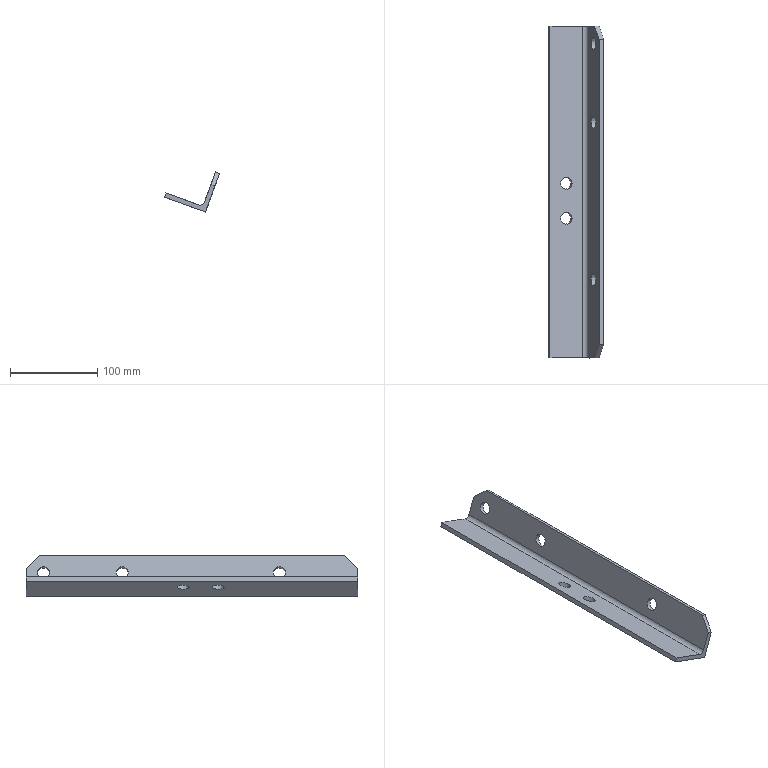Part | NX | features solid 2 | 1 solid | 16 faces | box 63.06 x 380 x 45.876 mm | volume 171865 mm3 | plane 10 | cylinder 6 | commonest cylinder face diameters 14 x5 10 x1
STEP:
#1=CARTESIAN_POINT('',(-698.232,780.,85.667));
#2=VERTEX_POINT('',#1);
#3=CARTESIAN_POINT('',(-695.838,780.,92.245));
#4=DIRECTION('',(-0.9397,0.,0.342));
#5=DIRECTION('',(-0.342,0.,-0.9397));
#6=AXIS2_PLACEMENT_3D('',#3,#4,#5);
#7=CIRCLE('',#6,7.);
#8=EDGE_CURVE('',#2,#2,#7,.F.);
#9=ORIENTED_EDGE('',*,*,#8,.T.);
#10=EDGE_LOOP('',(#9));
#11=FACE_BOUND('',#10,.T.);
#12=CARTESIAN_POINT('',(-698.232,960.,85.667));
#13=VERTEX_POINT('',#12);
#14=CARTESIAN_POINT('',(-695.838,960.,92.245));
#15=DIRECTION('',(-0.9397,0.,0.342));
#16=DIRECTION('',(-0.342,0.,-0.9397));
#17=AXIS2_PLACEMENT_3D('',#14,#15,#16);
#18=CIRCLE('',#17,7.);
#19=EDGE_CURVE('',#13,#13,#18,.F.);
#20=ORIENTED_EDGE('',*,*,#19,.T.);
#21=EDGE_LOOP('',(#20));
#22=FACE_BOUND('',#21,.T.);
#23=CARTESIAN_POINT('',(-694.127,1070.,96.944));
#24=VERTEX_POINT('',#23);
#25=CARTESIAN_POINT('',(-701.652,1070.,76.27));
#26=VERTEX_POINT('',#25);
#27=CARTESIAN_POINT('',(-693.101,1070.,99.763));
#28=DIRECTION('',(-0.342,0.,-0.9397));
#29=VECTOR('',#28,1000.);
#30=LINE('',#27,#29);
#31=EDGE_CURVE('',#24,#26,#30,.T.);
#32=ORIENTED_EDGE('',*,*,#31,.T.);
#33=CARTESIAN_POINT('',(-701.652,690.,76.27));
#34=VERTEX_POINT('',#33);
#35=CARTESIAN_POINT('',(-701.652,1109.813,76.27));
#36=DIRECTION('',(0.,1.,0.));
#37=VECTOR('',#36,1000.);
#38=LINE('',#35,#37);
#39=EDGE_CURVE('',#34,#26,#38,.T.);
#40=ORIENTED_EDGE('',*,*,#39,.F.);
#41=CARTESIAN_POINT('',(-694.127,690.,96.944));
#42=VERTEX_POINT('',#41);
#43=CARTESIAN_POINT('',(-695.838,690.,92.245));
#44=DIRECTION('',(0.342,0.,0.9397));
#45=VECTOR('',#44,1000.);
#46=LINE('',#43,#45);
#47=EDGE_CURVE('',#34,#42,#46,.T.);
#48=ORIENTED_EDGE('',*,*,#47,.T.);
#49=CARTESIAN_POINT('',(-688.997,705.,111.039));
#50=VERTEX_POINT('',#49);
#51=CARTESIAN_POINT('',(-670.59,758.818,161.611));
#52=DIRECTION('',(0.2418,0.7071,0.6645));
#53=VECTOR('',#52,1000.);
#54=LINE('',#51,#53);
#55=EDGE_CURVE('',#50,#42,#54,.F.);
#56=ORIENTED_EDGE('',*,*,#55,.F.);
#57=CARTESIAN_POINT('',(-688.997,1055.,111.039));
#58=VERTEX_POINT('',#57);
#59=CARTESIAN_POINT('',(-688.997,894.636,111.039));
#60=DIRECTION('',(0.,1.,0.));
#61=VECTOR('',#60,1000.);
#62=LINE('',#59,#61);
#63=EDGE_CURVE('',#50,#58,#62,.T.);
#64=ORIENTED_EDGE('',*,*,#63,.T.);
#65=CARTESIAN_POINT('',(-663.625,980.818,180.748));
#66=DIRECTION('',(0.2418,-0.7071,0.6645));
#67=VECTOR('',#66,1000.);
#68=LINE('',#65,#67);
#69=EDGE_CURVE('',#24,#58,#68,.T.);
#70=ORIENTED_EDGE('',*,*,#69,.F.);
#71=EDGE_LOOP('',(#32,#40,#48,#56,#64,#70));
#72=FACE_BOUND('',#71,.T.);
#73=CARTESIAN_POINT('',(-693.443,1050.,98.823));
#74=VERTEX_POINT('',#73);
#75=CARTESIAN_POINT('',(-695.838,1050.,92.245));
#76=DIRECTION('',(0.9397,0.,-0.342));
#77=DIRECTION('',(0.342,0.,0.9397));
#78=AXIS2_PLACEMENT_3D('',#75,#76,#77);
#79=CIRCLE('',#78,7.);
#80=EDGE_CURVE('',#74,#74,#79,.F.);
#81=ORIENTED_EDGE('',*,*,#80,.F.);
#82=EDGE_LOOP('',(#81));
#83=FACE_BOUND('',#82,.T.);
#84=CARTESIAN_POINT('',(-693.101,894.636,99.763));
#85=DIRECTION('',(-0.9397,0.,0.342));
#86=DIRECTION('',(-0.342,0.,-0.9397));
#87=AXIS2_PLACEMENT_3D('',#84,#85,#86);
#88=PLANE('',#87);
#89=ADVANCED_FACE('',(#11,#22,#72,#83),#88,.T.);
#90=CARTESIAN_POINT('',(-688.745,780.,97.113));
#91=VERTEX_POINT('',#90);
#92=CARTESIAN_POINT('',(-691.139,780.,90.535));
#93=DIRECTION('',(0.9397,0.,-0.342));
#94=DIRECTION('',(0.342,0.,0.9397));
#95=AXIS2_PLACEMENT_3D('',#92,#93,#94);
#96=CIRCLE('',#95,7.);
#97=EDGE_CURVE('',#91,#91,#96,.F.);
#98=ORIENTED_EDGE('',*,*,#97,.T.);
#99=EDGE_LOOP('',(#98));
#100=FACE_BOUND('',#99,.T.);
#101=CARTESIAN_POINT('',(-688.745,960.,97.113));
#102=VERTEX_POINT('',#101);
#103=CARTESIAN_POINT('',(-691.139,960.,90.535));
#104=DIRECTION('',(0.9397,0.,-0.342));
#105=DIRECTION('',(0.342,0.,0.9397));
#106=AXIS2_PLACEMENT_3D('',#103,#104,#105);
#107=CIRCLE('',#106,7.);
#108=EDGE_CURVE('',#102,#102,#107,.F.);
#109=ORIENTED_EDGE('',*,*,#108,.T.);
#110=EDGE_LOOP('',(#109));
#111=FACE_BOUND('',#110,.T.);
#112=CARTESIAN_POINT('',(-684.299,705.,109.329));
#113=VERTEX_POINT('',#112);
#114=CARTESIAN_POINT('',(-684.299,1055.,109.329));
#115=VERTEX_POINT('',#114);
#116=CARTESIAN_POINT('',(-684.299,894.636,109.329));
#117=DIRECTION('',(0.,1.,0.));
#118=VECTOR('',#117,1000.);
#119=LINE('',#116,#118);
#120=EDGE_CURVE('',#113,#115,#119,.T.);
#121=ORIENTED_EDGE('',*,*,#120,.F.);
#122=CARTESIAN_POINT('',(-689.429,690.,95.234));
#123=VERTEX_POINT('',#122);
#124=CARTESIAN_POINT('',(-665.892,758.818,159.901));
#125=DIRECTION('',(-0.2418,-0.7071,-0.6645));
#126=VECTOR('',#125,1000.);
#127=LINE('',#124,#126);
#128=EDGE_CURVE('',#123,#113,#127,.F.);
#129=ORIENTED_EDGE('',*,*,#128,.F.);
#130=CARTESIAN_POINT('',(-700.374,690.,65.163));
#131=VERTEX_POINT('',#130);
#132=CARTESIAN_POINT('',(-691.139,690.,90.535));
#133=DIRECTION('',(-0.342,0.,-0.9397));
#134=VECTOR('',#133,1000.);
#135=LINE('',#132,#134);
#136=EDGE_CURVE('',#123,#131,#135,.T.);
#137=ORIENTED_EDGE('',*,*,#136,.T.);
#138=CARTESIAN_POINT('',(-700.374,1070.,65.163));
#139=VERTEX_POINT('',#138);
#140=CARTESIAN_POINT('',(-700.374,894.636,65.163));
#141=DIRECTION('',(0.,1.,0.));
#142=VECTOR('',#141,1000.);
#143=LINE('',#140,#142);
#144=EDGE_CURVE('',#131,#139,#143,.T.);
#145=ORIENTED_EDGE('',*,*,#144,.T.);
#146=CARTESIAN_POINT('',(-689.429,1070.,95.234));
#147=VERTEX_POINT('',#146);
#148=CARTESIAN_POINT('',(-688.403,1070.,98.053));
#149=DIRECTION('',(0.342,0.,0.9397));
#150=VECTOR('',#149,1000.);
#151=LINE('',#148,#150);
#152=EDGE_CURVE('',#139,#147,#151,.T.);
#153=ORIENTED_EDGE('',*,*,#152,.T.);
#154=CARTESIAN_POINT('',(-658.927,980.818,179.037));
#155=DIRECTION('',(-0.2418,0.7071,-0.6645));
#156=VECTOR('',#155,1000.);
#157=LINE('',#154,#156);
#158=EDGE_CURVE('',#115,#147,#157,.T.);
#159=ORIENTED_EDGE('',*,*,#158,.F.);
#160=EDGE_LOOP('',(#121,#129,#137,#145,#153,#159));
#161=FACE_BOUND('',#160,.T.);
#162=CARTESIAN_POINT('',(-693.533,1050.,83.957));
#163=VERTEX_POINT('',#162);
#164=CARTESIAN_POINT('',(-691.139,1050.,90.535));
#165=DIRECTION('',(-0.9397,0.,0.342));
#166=DIRECTION('',(-0.342,0.,-0.9397));
#167=AXIS2_PLACEMENT_3D('',#164,#165,#166);
#168=CIRCLE('',#167,7.);
#169=EDGE_CURVE('',#163,#163,#168,.T.);
#170=ORIENTED_EDGE('',*,*,#169,.T.);
#171=EDGE_LOOP('',(#170));
#172=FACE_BOUND('',#171,.T.);
#173=CARTESIAN_POINT('',(-688.403,894.636,98.053));
#174=DIRECTION('',(0.9397,0.,-0.342));
#175=DIRECTION('',(0.342,0.,0.9397));
#176=AXIS2_PLACEMENT_3D('',#173,#174,#175);
#177=PLANE('',#176);
#178=ADVANCED_FACE('',(#100,#111,#161,#172),#177,.T.);
#179=ORIENTED_EDGE('',*,*,#63,.F.);
#180=CARTESIAN_POINT('',(-693.696,705.,112.749));
#181=DIRECTION('',(-0.9397,0.,0.342));
#182=VECTOR('',#181,1000.);
#183=LINE('',#180,#182);
#184=EDGE_CURVE('',#113,#50,#183,.T.);
#185=ORIENTED_EDGE('',*,*,#184,.F.);
#186=ORIENTED_EDGE('',*,*,#120,.T.);
#187=CARTESIAN_POINT('',(-684.299,1055.,109.329));
#188=DIRECTION('',(0.9397,0.,-0.342));
#189=VECTOR('',#188,1000.);
#190=LINE('',#187,#189);
#191=EDGE_CURVE('',#58,#115,#190,.T.);
#192=ORIENTED_EDGE('',*,*,#191,.F.);
#193=EDGE_LOOP('',(#179,#185,#186,#192));
#194=FACE_BOUND('',#193,.T.);
#195=CARTESIAN_POINT('',(-693.696,894.636,112.749));
#196=DIRECTION('',(0.342,0.,0.9397));
#197=DIRECTION('',(0.,1.,0.));
#198=AXIS2_PLACEMENT_3D('',#195,#196,#197);
#199=PLANE('',#198);
#200=ADVANCED_FACE('',(#194),#199,.T.);
#201=CARTESIAN_POINT('',(-708.06,1070.,73.282));
#202=VERTEX_POINT('',#201);
#203=CARTESIAN_POINT('',(-708.06,690.,73.282));
#204=VERTEX_POINT('',#203);
#205=CARTESIAN_POINT('',(-708.06,775.,73.282));
#206=DIRECTION('',(0.,1.,0.));
#207=VECTOR('',#206,1000.);
#208=LINE('',#205,#207);
#209=EDGE_CURVE('',#202,#204,#208,.F.);
#210=ORIENTED_EDGE('',*,*,#209,.T.);
#211=CARTESIAN_POINT('',(-706.35,690.,77.981));
#212=DIRECTION('',(0.,1.,0.));
#213=DIRECTION('',(-0.9962,0.,-0.08716));
#214=AXIS2_PLACEMENT_3D('',#211,#212,#213);
#215=CIRCLE('',#214,5.);
#216=EDGE_CURVE('',#34,#204,#215,.T.);
#217=ORIENTED_EDGE('',*,*,#216,.F.);
#218=ORIENTED_EDGE('',*,*,#39,.T.);
#219=CARTESIAN_POINT('',(-706.35,1070.,77.981));
#220=DIRECTION('',(0.,1.,0.));
#221=DIRECTION('',(-0.08716,0.,0.9962));
#222=AXIS2_PLACEMENT_3D('',#219,#220,#221);
#223=CIRCLE('',#222,5.);
#224=EDGE_CURVE('',#202,#26,#223,.F.);
#225=ORIENTED_EDGE('',*,*,#224,.F.);
#226=EDGE_LOOP('',(#210,#217,#218,#225));
#227=FACE_BOUND('',#226,.T.);
#228=CARTESIAN_POINT('',(-706.35,894.636,77.981));
#229=DIRECTION('',(0.,-1.,0.));
#230=DIRECTION('',(-0.342,0.,-0.9397));
#231=AXIS2_PLACEMENT_3D('',#228,#229,#230);
#232=CYLINDRICAL_SURFACE('',#231,5.);
#233=ADVANCED_FACE('',(#227),#232,.F.);
#234=CARTESIAN_POINT('',(-745.648,1070.,86.963));
#235=VERTEX_POINT('',#234);
#236=CARTESIAN_POINT('',(-747.358,1070.,82.264));
#237=VERTEX_POINT('',#236);
#238=CARTESIAN_POINT('',(-735.388,1070.,115.154));
#239=DIRECTION('',(-0.342,0.,-0.9397));
#240=VECTOR('',#239,1000.);
#241=LINE('',#238,#240);
#242=EDGE_CURVE('',#235,#237,#241,.T.);
#243=ORIENTED_EDGE('',*,*,#242,.T.);
#244=CARTESIAN_POINT('',(-747.358,690.,82.264));
#245=VERTEX_POINT('',#244);
#246=CARTESIAN_POINT('',(-747.358,892.5,82.264));
#247=DIRECTION('',(0.,1.,0.));
#248=VECTOR('',#247,1000.);
#249=LINE('',#246,#248);
#250=EDGE_CURVE('',#245,#237,#249,.T.);
#251=ORIENTED_EDGE('',*,*,#250,.F.);
#252=CARTESIAN_POINT('',(-745.648,690.,86.963));
#253=VERTEX_POINT('',#252);
#254=CARTESIAN_POINT('',(-738.124,690.,107.636));
#255=DIRECTION('',(0.342,0.,0.9397));
#256=VECTOR('',#255,1000.);
#257=LINE('',#254,#256);
#258=EDGE_CURVE('',#245,#253,#257,.T.);
#259=ORIENTED_EDGE('',*,*,#258,.T.);
#260=CARTESIAN_POINT('',(-745.648,894.636,86.963));
#261=DIRECTION('',(0.,1.,0.));
#262=VECTOR('',#261,1000.);
#263=LINE('',#260,#262);
#264=EDGE_CURVE('',#253,#235,#263,.T.);
#265=ORIENTED_EDGE('',*,*,#264,.T.);
#266=EDGE_LOOP('',(#243,#251,#259,#265));
#267=FACE_BOUND('',#266,.T.);
#268=CARTESIAN_POINT('',(-735.388,894.636,115.154));
#269=DIRECTION('',(-0.9397,0.,0.342));
#270=DIRECTION('',(-0.342,0.,-0.9397));
#271=AXIS2_PLACEMENT_3D('',#268,#269,#270);
#272=PLANE('',#271);
#273=ADVANCED_FACE('',(#267),#272,.T.);
#274=CARTESIAN_POINT('',(-733.432,850.,82.517));
#275=VERTEX_POINT('',#274);
#276=CARTESIAN_POINT('',(-726.854,850.,80.122));
#277=DIRECTION('',(0.342,0.,0.9397));
#278=DIRECTION('',(-0.9397,0.,0.342));
#279=AXIS2_PLACEMENT_3D('',#276,#277,#278);
#280=CIRCLE('',#279,7.);
#281=EDGE_CURVE('',#275,#275,#280,.T.);
#282=ORIENTED_EDGE('',*,*,#281,.F.);
#283=EDGE_LOOP('',(#282));
#284=FACE_BOUND('',#283,.T.);
#285=CARTESIAN_POINT('',(-733.432,890.,82.517));
#286=VERTEX_POINT('',#285);
#287=CARTESIAN_POINT('',(-726.854,890.,80.122));
#288=DIRECTION('',(0.342,0.,0.9397));
#289=DIRECTION('',(-0.9397,0.,0.342));
#290=AXIS2_PLACEMENT_3D('',#287,#288,#289);
#291=CIRCLE('',#290,7.);
#292=EDGE_CURVE('',#286,#286,#291,.T.);
#293=ORIENTED_EDGE('',*,*,#292,.F.);
#294=EDGE_LOOP('',(#293));
#295=FACE_BOUND('',#294,.T.);
#296=CARTESIAN_POINT('',(-745.648,1070.,86.963));
#297=DIRECTION('',(-0.9397,0.,0.342));
#298=VECTOR('',#297,1000.);
#299=LINE('',#296,#298);
#300=EDGE_CURVE('',#202,#235,#299,.T.);
#301=ORIENTED_EDGE('',*,*,#300,.T.);
#302=ORIENTED_EDGE('',*,*,#264,.F.);
#303=CARTESIAN_POINT('',(-703.362,690.,71.572));
#304=DIRECTION('',(0.9397,0.,-0.342));
#305=VECTOR('',#304,1000.);
#306=LINE('',#303,#305);
#307=EDGE_CURVE('',#253,#204,#306,.T.);
#308=ORIENTED_EDGE('',*,*,#307,.T.);
#309=ORIENTED_EDGE('',*,*,#209,.F.);
#310=EDGE_LOOP('',(#301,#302,#308,#309));
#311=FACE_BOUND('',#310,.T.);
#312=CARTESIAN_POINT('',(-745.648,892.805,86.963));
#313=DIRECTION('',(0.342,0.,0.9397));
#314=DIRECTION('',(0.,1.,0.));
#315=AXIS2_PLACEMENT_3D('',#312,#313,#314);
#316=PLANE('',#315);
#317=ADVANCED_FACE('',(#284,#295,#311),#316,.T.);
#318=CARTESIAN_POINT('',(-735.142,850.,77.818));
#319=VERTEX_POINT('',#318);
#320=CARTESIAN_POINT('',(-728.564,850.,75.424));
#321=DIRECTION('',(0.342,0.,0.9397));
#322=DIRECTION('',(-0.9397,0.,0.342));
#323=AXIS2_PLACEMENT_3D('',#320,#321,#322);
#324=CIRCLE('',#323,7.);
#325=EDGE_CURVE('',#319,#319,#324,.T.);
#326=ORIENTED_EDGE('',*,*,#325,.T.);
#327=EDGE_LOOP('',(#326));
#328=FACE_BOUND('',#327,.T.);
#329=CARTESIAN_POINT('',(-735.142,890.,77.818));
#330=VERTEX_POINT('',#329);
#331=CARTESIAN_POINT('',(-728.564,890.,75.424));
#332=DIRECTION('',(0.342,0.,0.9397));
#333=DIRECTION('',(-0.9397,0.,0.342));
#334=AXIS2_PLACEMENT_3D('',#331,#332,#333);
#335=CIRCLE('',#334,7.);
#336=EDGE_CURVE('',#330,#330,#335,.T.);
#337=ORIENTED_EDGE('',*,*,#336,.T.);
#338=EDGE_LOOP('',(#337));
#339=FACE_BOUND('',#338,.T.);
#340=CARTESIAN_POINT('',(-705.072,1070.,66.874));
#341=DIRECTION('',(0.9397,0.,-0.342));
#342=VECTOR('',#341,1000.);
#343=LINE('',#340,#342);
#344=EDGE_CURVE('',#237,#139,#343,.T.);
#345=ORIENTED_EDGE('',*,*,#344,.T.);
#346=ORIENTED_EDGE('',*,*,#144,.F.);
#347=CARTESIAN_POINT('',(-705.072,690.,66.874));
#348=DIRECTION('',(-0.9397,0.,0.342));
#349=VECTOR('',#348,1000.);
#350=LINE('',#347,#349);
#351=EDGE_CURVE('',#131,#245,#350,.T.);
#352=ORIENTED_EDGE('',*,*,#351,.T.);
#353=ORIENTED_EDGE('',*,*,#250,.T.);
#354=EDGE_LOOP('',(#345,#346,#352,#353));
#355=FACE_BOUND('',#354,.T.);
#356=CARTESIAN_POINT('',(-705.072,892.5,66.874));
#357=DIRECTION('',(-0.342,0.,-0.9397));
#358=DIRECTION('',(0.,-1.,0.));
#359=AXIS2_PLACEMENT_3D('',#356,#357,#358);
#360=PLANE('',#359);
#361=ADVANCED_FACE('',(#328,#339,#355),#360,.T.);
#362=ORIENTED_EDGE('',*,*,#19,.F.);
#363=EDGE_LOOP('',(#362));
#364=FACE_BOUND('',#363,.T.);
#365=ORIENTED_EDGE('',*,*,#108,.F.);
#366=EDGE_LOOP('',(#365));
#367=FACE_BOUND('',#366,.T.);
#368=CARTESIAN_POINT('',(-719.33,960.,100.796));
#369=DIRECTION('',(0.9397,0.,-0.342));
#370=DIRECTION('',(0.,1.,0.));
#371=AXIS2_PLACEMENT_3D('',#368,#369,#370);
#372=CYLINDRICAL_SURFACE('',#371,7.);
#373=ADVANCED_FACE('',(#364,#367),#372,.F.);
#374=ORIENTED_EDGE('',*,*,#152,.F.);
#375=ORIENTED_EDGE('',*,*,#344,.F.);
#376=ORIENTED_EDGE('',*,*,#242,.F.);
#377=ORIENTED_EDGE('',*,*,#300,.F.);
#378=ORIENTED_EDGE('',*,*,#224,.T.);
#379=ORIENTED_EDGE('',*,*,#31,.F.);
#380=CARTESIAN_POINT('',(-694.127,1070.,96.944));
#381=DIRECTION('',(-0.9397,0.,0.342));
#382=VECTOR('',#381,1000.);
#383=LINE('',#380,#382);
#384=EDGE_CURVE('',#147,#24,#383,.T.);
#385=ORIENTED_EDGE('',*,*,#384,.F.);
#386=EDGE_LOOP('',(#374,#375,#376,#377,#378,#379,#385));
#387=FACE_BOUND('',#386,.T.);
#388=CARTESIAN_POINT('',(-118.087,1070.,-25.569));
#389=DIRECTION('',(0.,-1.,0.));
#390=DIRECTION('',(-0.08716,0.,0.9962));
#391=AXIS2_PLACEMENT_3D('',#388,#389,#390);
#392=PLANE('',#391);
#393=ADVANCED_FACE('',(#387),#392,.F.);
#394=ORIENTED_EDGE('',*,*,#47,.F.);
#395=ORIENTED_EDGE('',*,*,#216,.T.);
#396=ORIENTED_EDGE('',*,*,#307,.F.);
#397=ORIENTED_EDGE('',*,*,#258,.F.);
#398=ORIENTED_EDGE('',*,*,#351,.F.);
#399=ORIENTED_EDGE('',*,*,#136,.F.);
#400=CARTESIAN_POINT('',(-694.127,690.,96.944));
#401=DIRECTION('',(0.9397,0.,-0.342));
#402=VECTOR('',#401,1000.);
#403=LINE('',#400,#402);
#404=EDGE_CURVE('',#42,#123,#403,.T.);
#405=ORIENTED_EDGE('',*,*,#404,.F.);
#406=EDGE_LOOP('',(#394,#395,#396,#397,#398,#399,#405));
#407=FACE_BOUND('',#406,.T.);
#408=CARTESIAN_POINT('',(-695.838,690.,92.245));
#409=DIRECTION('',(0.,-1.,0.));
#410=DIRECTION('',(0.7071,0.,-0.7071));
#411=AXIS2_PLACEMENT_3D('',#408,#409,#410);
#412=PLANE('',#411);
#413=ADVANCED_FACE('',(#407),#412,.T.);
#414=ORIENTED_EDGE('',*,*,#8,.F.);
#415=EDGE_LOOP('',(#414));
#416=FACE_BOUND('',#415,.T.);
#417=ORIENTED_EDGE('',*,*,#97,.F.);
#418=EDGE_LOOP('',(#417));
#419=FACE_BOUND('',#418,.T.);
#420=CARTESIAN_POINT('',(-719.33,780.,100.796));
#421=DIRECTION('',(0.9397,0.,-0.342));
#422=DIRECTION('',(0.,1.,0.));
#423=AXIS2_PLACEMENT_3D('',#420,#421,#422);
#424=CYLINDRICAL_SURFACE('',#423,7.);
#425=ADVANCED_FACE('',(#416,#419),#424,.F.);
#426=ORIENTED_EDGE('',*,*,#80,.T.);
#427=EDGE_LOOP('',(#426));
#428=FACE_BOUND('',#427,.T.);
#429=ORIENTED_EDGE('',*,*,#169,.F.);
#430=EDGE_LOOP('',(#429));
#431=FACE_BOUND('',#430,.T.);
#432=CARTESIAN_POINT('',(-719.33,1050.,100.796));
#433=DIRECTION('',(0.9397,0.,-0.342));
#434=DIRECTION('',(0.,1.,0.));
#435=AXIS2_PLACEMENT_3D('',#432,#433,#434);
#436=CYLINDRICAL_SURFACE('',#435,7.);
#437=ADVANCED_FACE('',(#428,#431),#436,.F.);
#438=ORIENTED_EDGE('',*,*,#158,.T.);
#439=ORIENTED_EDGE('',*,*,#384,.T.);
#440=ORIENTED_EDGE('',*,*,#69,.T.);
#441=ORIENTED_EDGE('',*,*,#191,.T.);
#442=EDGE_LOOP('',(#438,#439,#440,#441));
#443=FACE_BOUND('',#442,.T.);
#444=CARTESIAN_POINT('',(-146.096,1070.,-102.524));
#445=DIRECTION('',(0.2418,0.7071,0.6645));
#446=DIRECTION('',(0.06458,0.6715,-0.7381));
#447=AXIS2_PLACEMENT_3D('',#444,#445,#446);
#448=PLANE('',#447);
#449=ADVANCED_FACE('',(#443),#448,.T.);
#450=ORIENTED_EDGE('',*,*,#55,.T.);
#451=ORIENTED_EDGE('',*,*,#404,.T.);
#452=ORIENTED_EDGE('',*,*,#128,.T.);
#453=ORIENTED_EDGE('',*,*,#184,.T.);
#454=EDGE_LOOP('',(#450,#451,#452,#453));
#455=FACE_BOUND('',#454,.T.);
#456=CARTESIAN_POINT('',(-694.127,690.,96.944));
#457=DIRECTION('',(-0.2418,0.7071,-0.6645));
#458=DIRECTION('',(0.06458,-0.6715,-0.7381));
#459=AXIS2_PLACEMENT_3D('',#456,#457,#458);
#460=PLANE('',#459);
#461=ADVANCED_FACE('',(#455),#460,.F.);
#462=ORIENTED_EDGE('',*,*,#336,.F.);
#463=EDGE_LOOP('',(#462));
#464=FACE_BOUND('',#463,.T.);
#465=ORIENTED_EDGE('',*,*,#292,.T.);
#466=EDGE_LOOP('',(#465));
#467=FACE_BOUND('',#466,.T.);
#468=CARTESIAN_POINT('',(-726.854,890.,80.122));
#469=DIRECTION('',(-0.342,0.,-0.9397));
#470=DIRECTION('',(-0.9397,0.,0.342));
#471=AXIS2_PLACEMENT_3D('',#468,#469,#470);
#472=CYLINDRICAL_SURFACE('',#471,7.);
#473=ADVANCED_FACE('',(#464,#467),#472,.F.);
#474=ORIENTED_EDGE('',*,*,#325,.F.);
#475=EDGE_LOOP('',(#474));
#476=FACE_BOUND('',#475,.T.);
#477=ORIENTED_EDGE('',*,*,#281,.T.);
#478=EDGE_LOOP('',(#477));
#479=FACE_BOUND('',#478,.T.);
#480=CARTESIAN_POINT('',(-726.854,850.,80.122));
#481=DIRECTION('',(-0.342,0.,-0.9397));
#482=DIRECTION('',(-0.9397,0.,0.342));
#483=AXIS2_PLACEMENT_3D('',#480,#481,#482);
#484=CYLINDRICAL_SURFACE('',#483,7.);
#485=ADVANCED_FACE('',(#476,#479),#484,.F.);
#486=CLOSED_SHELL('',(#89,#178,#200,#233,#273,#317,#361,#373,#393,#413,#425,#437,#449,#461,#473,#485));
#487=MANIFOLD_SOLID_BREP('',#486);
#488=(LENGTH_UNIT()NAMED_UNIT(*)SI_UNIT(.MILLI.,.METRE.));
#489=UNCERTAINTY_MEASURE_WITH_UNIT(LENGTH_MEASURE(0.00001),#488,'','');
#490=(NAMED_UNIT(*)PLANE_ANGLE_UNIT()SI_UNIT($,.RADIAN.));
#491=(NAMED_UNIT(*)SI_UNIT($,.STERADIAN.)SOLID_ANGLE_UNIT());
#492=(GEOMETRIC_REPRESENTATION_CONTEXT(3)GLOBAL_UNCERTAINTY_ASSIGNED_CONTEXT((#489))GLOBAL_UNIT_ASSIGNED_CONTEXT((#488,#490,#491))REPRESENTATION_CONTEXT('',''));
#493=ADVANCED_BREP_SHAPE_REPRESENTATION('',(#487),#492);